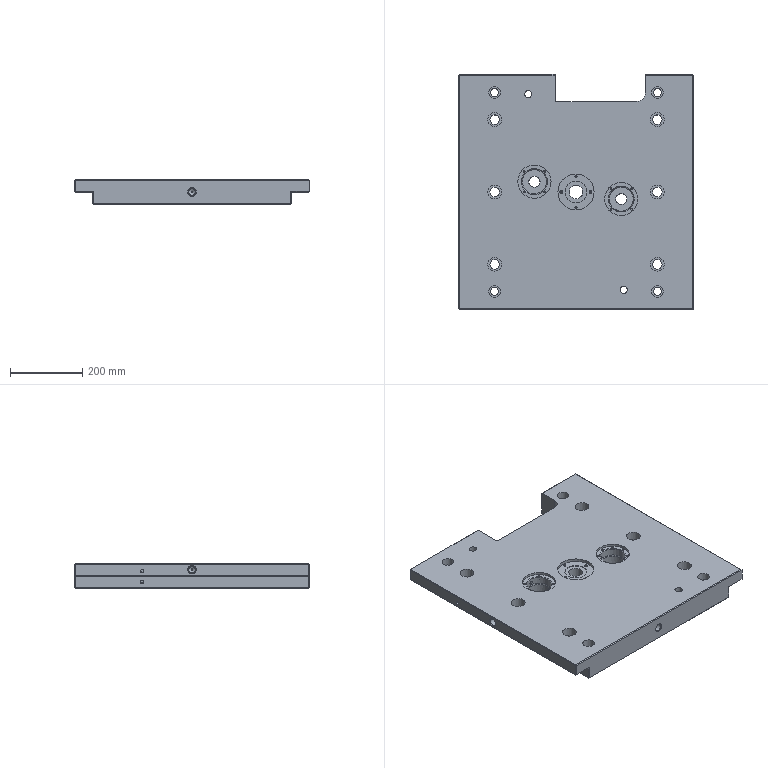Part | STEP file | P011002A004-000 | 1 solid | 1171 faces | box 650 x 650 x 70 mm | volume 24694977 mm3 | plane 740 | other 157 | cone 153 | cylinder 119 | torus 2 | commonest cylinder face diameters 5 x18 8 x16 4.167 x14 4.983 x14 6 x9 38 x7